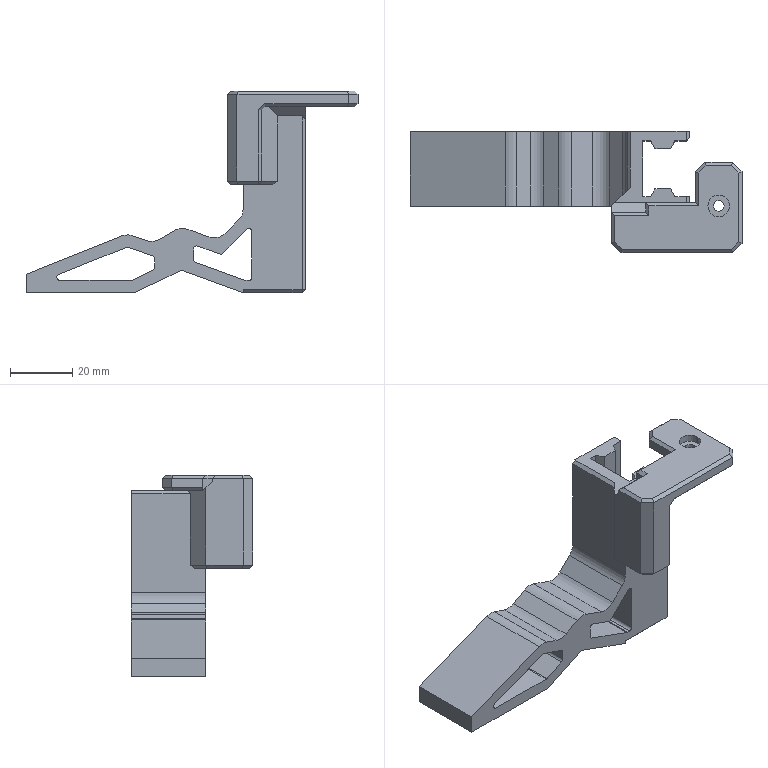Part | SolidWorks | features ICE 7, Chamfer 6, Fillet 2, 3DProfileFeature 1, Extrusion 1, HoleWzd 1 | 1 solid | 124 faces | box 107 x 39 x 65 mm | volume 37436 mm3 | plane 104 | cylinder 20 | commonest cylinder face diameters 2 x11 10 x5 3.4 x2 7 x2